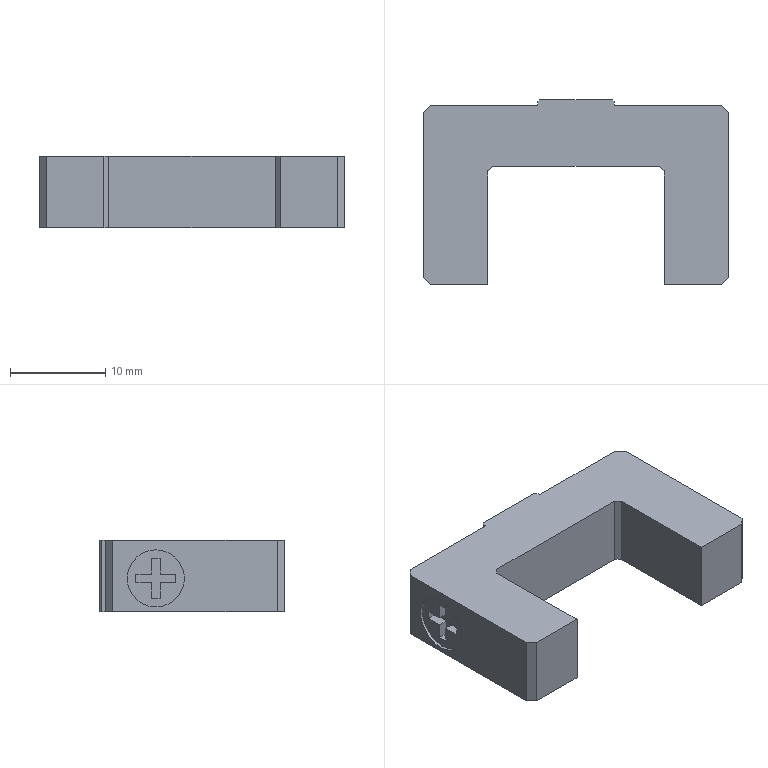Part | STEP file | 9 | 1 solid | 57 faces | box 32 x 19.4 x 7.5 mm | volume 2771 mm3 | plane 51 | cylinder 6 | commonest cylinder face diameters 6 x4 5 x2